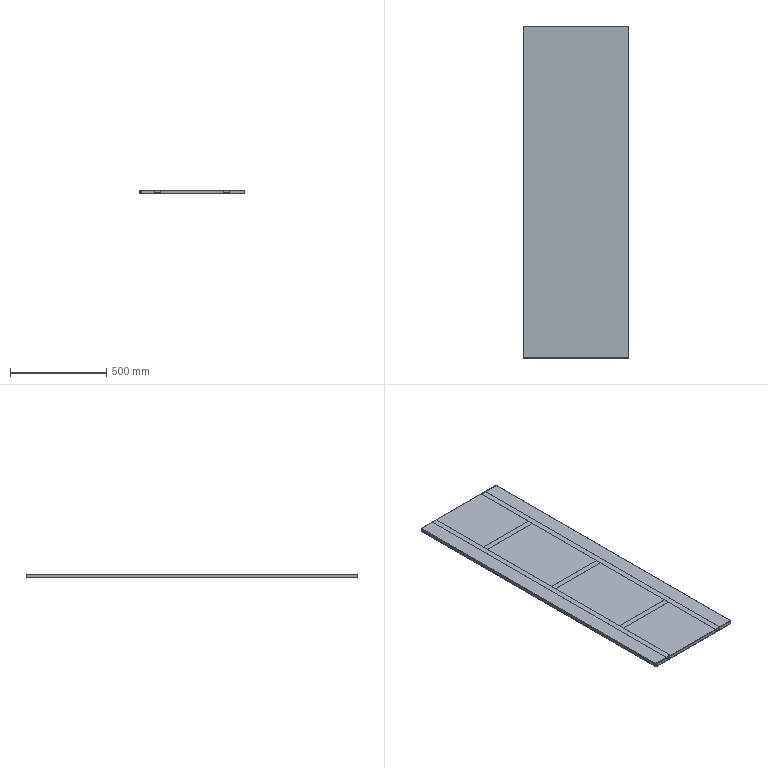Part | SolidWorks | features BaseBody 6 | 6 solids | 124 faces | box 549 x 1721 x 20 mm | volume 1317735 mm3 | plane 88 | cylinder 20 | spline 16 | commonest cylinder face diameters 2 x8 4 x8 8 x4